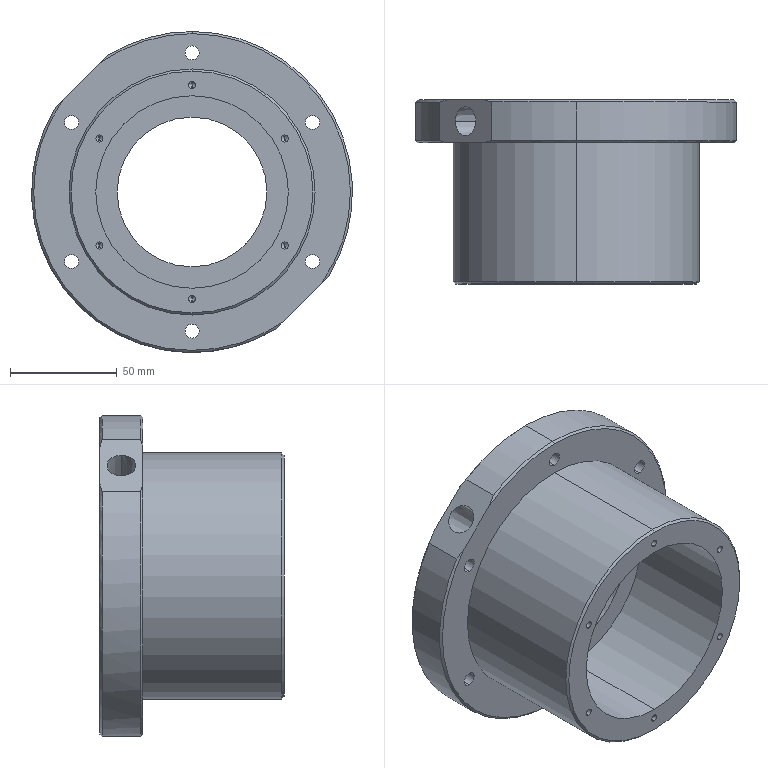Part | STEP file | 10-03 rotary bearing seat | 1 solid | 127 faces | box 150 x 86 x 150 mm | volume 549406 mm3 | cylinder 69 | cone 42 | plane 16 | commonest cylinder face diameters 3.3 x12 4.2 x12 6.6 x12 11 x12 10 x4 10.7 x4